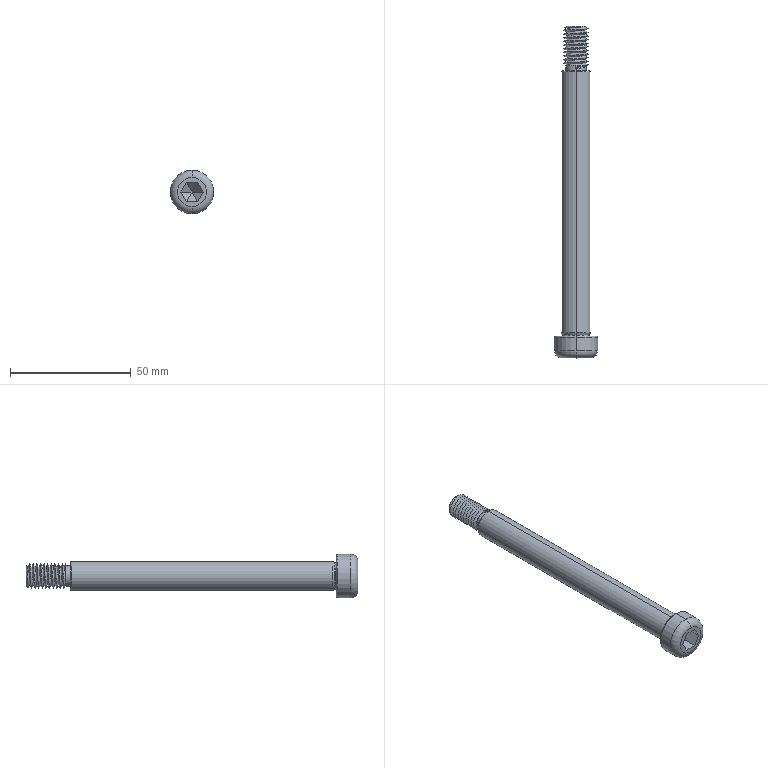Part | SolidWorks | features BaseBody 1 | 1 solid | 44 faces | box 18 x 137.5 x 18 mm | volume 15167 mm3 | plane 18 | torus 14 | cylinder 7 | cone 3 | spline 2 | commonest cylinder face diameters 8.5 x3 11.98 x2 18 x2